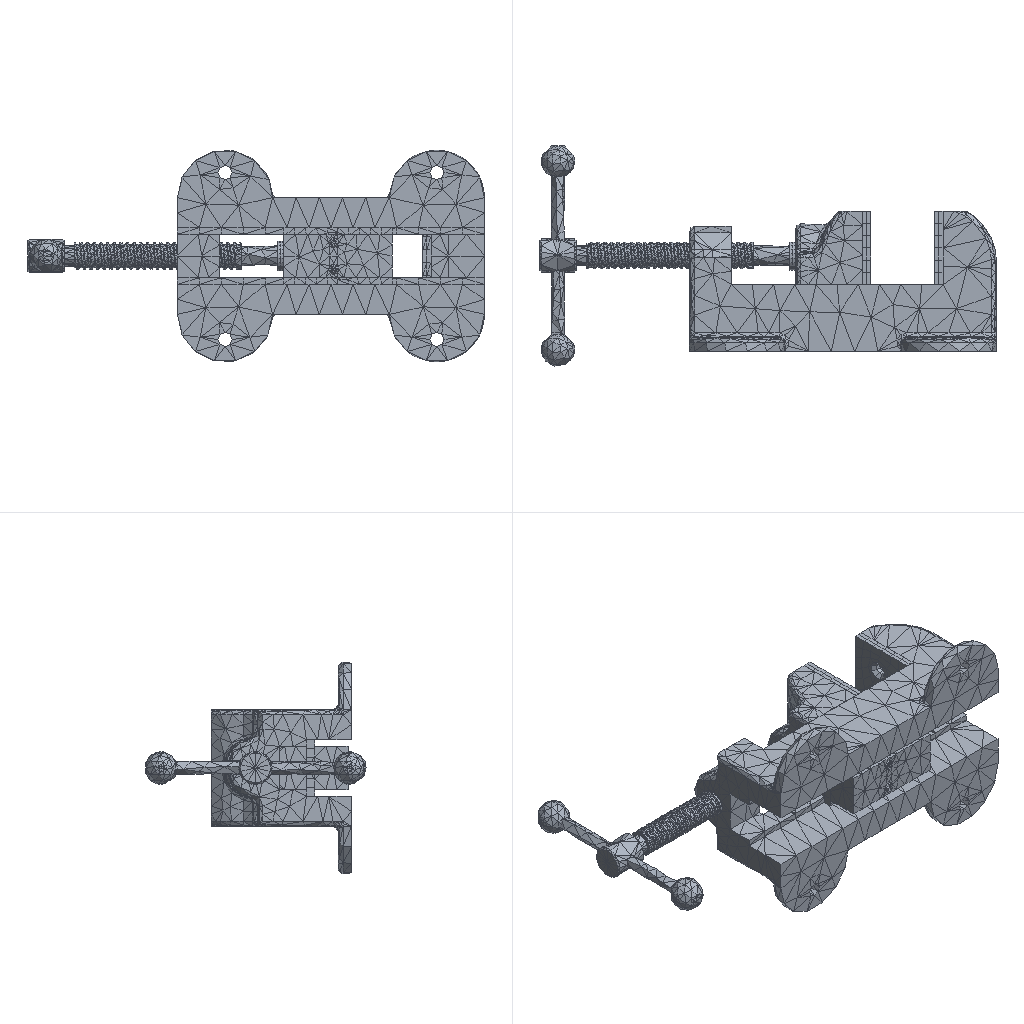Simulation study | ansys workbench
Set-up summary:
category,name,step,type,value,unit,region
solver,ansys_workbench
units,mm-N-s-tonne (MPa),,stated,"/units,MPA"
analysis,deck-1/LS1,,static
load_step,deck-1/LS1,deck-1/LS1,static,nsubst=1; time=1
analysis,deck-2/LS1,,static
load_step,deck-2/LS1,deck-2/LS1,static,nsubst=1; time=1
mesh,deck-1.dat,,nodes,53538
mesh,deck-1.dat,,elements,38064
element_type,SOLID187,,,25842,,deck-1.dat
element_type,TARGE170,,,5584,,deck-1.dat
element_type,CONTA174,,,5584,,deck-1.dat
element_type,SOLID186,,,872,,deck-1.dat
element_type,SURF154,,,182,,deck-1.dat
mesh,deck-2.dat,,nodes,49348
mesh,deck-2.dat,,elements,34462
element_type,SOLID187,,,24682,,deck-2.dat
element_type,TARGE170,,,4587,,deck-2.dat
element_type,CONTA174,,,4587,,deck-2.dat
element_type,SOLID186,,,442,,deck-2.dat
element_type,SURF154,,,164,,deck-2.dat
material,Q235,,E,200000,tonne s^-2 mm^-1
material,Q235,,nu,0.3
material,Q235,,density,7.85e-09,tonne mm^-3
material,Q235,,conductivity,60.5,tonne mm s^-3 C^-1
material,Q235,,specific_heat,4.34e+08,mm^2 s^-2 C^-1
material,Q235,,cte,1.2e-05,C^-1
material,Q235,,permeability,10000
material,Q235,,resistivity,0.00017,ohm mm
material,Structural Steel,,E,200000,tonne s^-2 mm^-1
material,Structural Steel,,nu,0.3
material,Structural Steel,,density,7.85e-09,tonne mm^-3
material,Structural Steel,,conductivity,60.5,tonne mm s^-3 C^-1
material,Structural Steel,,specific_heat,4.34e+08,mm^2 s^-2 C^-1
material,Structural Steel,,cte,1.2e-05,C^-1
material,Structural Steel,,permeability,10000
material,Structural Steel,,resistivity,0.00017,ohm mm
load,Define Force Using Surface Effect Elements,deck-1/LS1,surface-effect pres face 1,-1.743,,SURF154 #70
load,Define Force Using Surface Effect Elements,deck-1/LS1,surface-effect pres face 2,6.79742e-14,,SURF154 #70
load,Define Force Using Surface Effect Elements,deck-1/LS1,surface-effect pres face 3,6.97171e-15,,SURF154 #70
load,Define Force Using Surface Effect Elements,deck-1/LS1,surface-effect pres face 1,1.743,,SURF154 #71
load,Define Force Using Surface Effect Elements,deck-1/LS1,surface-effect pres face 3,6.97171e-15,,SURF154 #71
load,Define Force Using Surface Effect Elements,deck-1/LS1,surface-effect pres face 2,-0.8948,,SURF154 #72
load,Define Force Using Surface Effect Elements,deck-2/LS1,surface-effect pres face 1,-1.743,,SURF154 #70
load,Define Force Using Surface Effect Elements,deck-2/LS1,surface-effect pres face 2,6.79645e-14,,SURF154 #70
load,Define Force Using Surface Effect Elements,deck-2/LS1,surface-effect pres face 3,6.97071e-15,,SURF154 #70
load,Define Force Using Surface Effect Elements,deck-2/LS1,surface-effect pres face 1,1.743,,SURF154 #71
load,Define Force Using Surface Effect Elements,deck-2/LS1,surface-effect pres face 3,6.97071e-15,,SURF154 #71
load,Define Force Using Surface Effect Elements,deck-2/LS1,surface-effect pres face 2,-0.8948,,SURF154 #72
bc,Fixed Supports,deck-1/model,fixed,[dofs=ALL],,_FIXEDSU
bc,Fixed Supports,deck-2/model,fixed,[dofs=ALL],,_FIXEDSU
contact,Contact Region,,bonded (always),element=CONTA174
contact,Contact Region 2,,bonded (always),element=CONTA174
contact,Contact Region 3,,bonded (always),element=CONTA174
contact,Contact Region 4,,bonded (always),element=CONTA174
contact,Contact Region 5,,bonded (always),element=CONTA174
contact,Contact Region 6,,bonded (always),element=CONTA174
contact,Contact Region 7,,bonded (always),element=CONTA174
contact,Contact Region 8,,bonded (always),element=CONTA174
contact,Contact Region 9,,bonded (always),element=CONTA174
contact,Contact Region 10,,bonded (always),element=CONTA174
contact,Contact Region 11,,bonded (always),element=CONTA174
contact,Contact Region 12,,bonded (always),element=CONTA174
contact,Contact Region 13,,bonded (always),element=CONTA174
contact,Contact Region 14,,bonded (always),element=CONTA174
contact,Contact Region 15,,bonded (always),element=CONTA174
contact,Contact Region 16,,bonded (always),element=CONTA174
contact,Contact Region 17,,bonded (always),element=CONTA174
contact,Contact Region 18,,bonded (always),element=CONTA174
contact,Contact Region 19,,bonded (always),element=CONTA174
contact,Contact Region 20,,bonded (always),element=CONTA174
contact,Contact Region 21,,bonded (always),element=CONTA174
contact,Contact Region 22,,bonded (always),element=CONTA174
contact,Contact Region 23,,bonded (always),element=CONTA174
contact,Contact Region 24,,bonded (always),element=CONTA174
contact,Contact Region 25,,bonded (always),element=CONTA174
contact,Contact Region 26,,bonded (always),element=CONTA174
contact,Contact Region,,bonded (always),element=CONTA174
contact,Contact Region 2,,bonded (always),element=CONTA174
contact,Contact Region 3,,bonded (always),element=CONTA174
contact,Contact Region 4,,bonded (always),element=CONTA174
contact,Contact Region 5,,bonded (always),element=CONTA174
contact,Contact Region 6,,bonded (always),element=CONTA174
contact,Contact Region 7,,bonded (always),element=CONTA174
contact,Contact Region 8,,bonded (always),element=CONTA174
contact,Contact Region 9,,bonded (always),element=CONTA174
contact,Contact Region 10,,bonded (always),element=CONTA174
contact,Contact Region 11,,bonded (always),element=CONTA174
contact,Contact Region 12,,bonded (always),element=CONTA174
contact,Contact Region 13,,bonded (always),element=CONTA174
contact,Contact Region 14,,bonded (always),element=CONTA174
contact,Contact Region 15,,bonded (always),element=CONTA174
contact,Contact Region 16,,bonded (always),element=CONTA174
contact,Contact Region 17,,bonded (always),element=CONTA174
contact,Contact Region 18,,bonded (always),element=CONTA174
contact,Contact Region 19,,bonded (always),element=CONTA174
contact,Contact Region 20,,bonded (always),element=CONTA174
contact,Contact Region 21,,bonded (always),element=CONTA174
contact,Contact Region 22,,bonded (always),element=CONTA174
contact,Contact Region 23,,bonded (always),element=CONTA174
contact,Contact Region 24,,bonded (always),element=CONTA174
contact,Contact Region 25,,bonded (always),element=CONTA174
contact,Contact Region 26,,bonded (always),element=CONTA174
named_set,_FIXEDSU,,node,420
named_set,_FIXEDSU,,node,370
Results summary:
result,analyses[0].index,,,1
result,analyses[0].system,,,SYS
result,analyses[0].deck,,,deck-1.dat
result,analyses[0].solve_status,,,completed
result,analyses[0].analysis_type,,,static
result,analyses[0].physics,,,mechanical
result,analyses[0].unit_system,,,"NMM: mm, ton, N, s, mV, mA, degC"
result,analyses[0].n_sets,,,1
result,analyses[0].load_steps[0].set,set=1,,1
result,analyses[0].load_steps[0].time_or_freq,set=1,,1
result,analyses[0].load_steps[0].max_displacement_magnitude,set=1,,0.007504
result,analyses[0].load_steps[0].max_von_mises_nodal,set=1,,41.43
result,analyses[0].load_steps[0].reaction_force_sum_xyz[1],set=1,,-1.39599e-08
result,analyses[0].load_steps[0].reaction_force_sum_xyz[2],set=1,,5000
result,analyses[0].load_steps[0].reaction_force_sum_xyz[3],set=1,,1.51558e-08
result,analyses[1].index,,,2
result,analyses[1].system,,,SYS-1
result,analyses[1].deck,,,deck-2.dat
result,analyses[1].solve_status,,,completed
result,analyses[1].analysis_type,,,static
result,analyses[1].physics,,,mechanical
result,analyses[1].unit_system,,,"NMM: mm, ton, N, s, mV, mA, degC"
result,analyses[1].n_sets,,,1
result,analyses[1].load_steps[0].set,set=1,,1
result,analyses[1].load_steps[0].time_or_freq,set=1,,1
result,analyses[1].load_steps[0].max_displacement_magnitude,set=1,,0.01517
result,analyses[1].load_steps[0].max_von_mises_nodal,set=1,,56.068
result,analyses[1].load_steps[0].reaction_force_sum_xyz[1],set=1,,2.00742e-06
result,analyses[1].load_steps[0].reaction_force_sum_xyz[2],set=1,,5000
result,analyses[1].load_steps[0].reaction_force_sum_xyz[3],set=1,,2.63775e-06